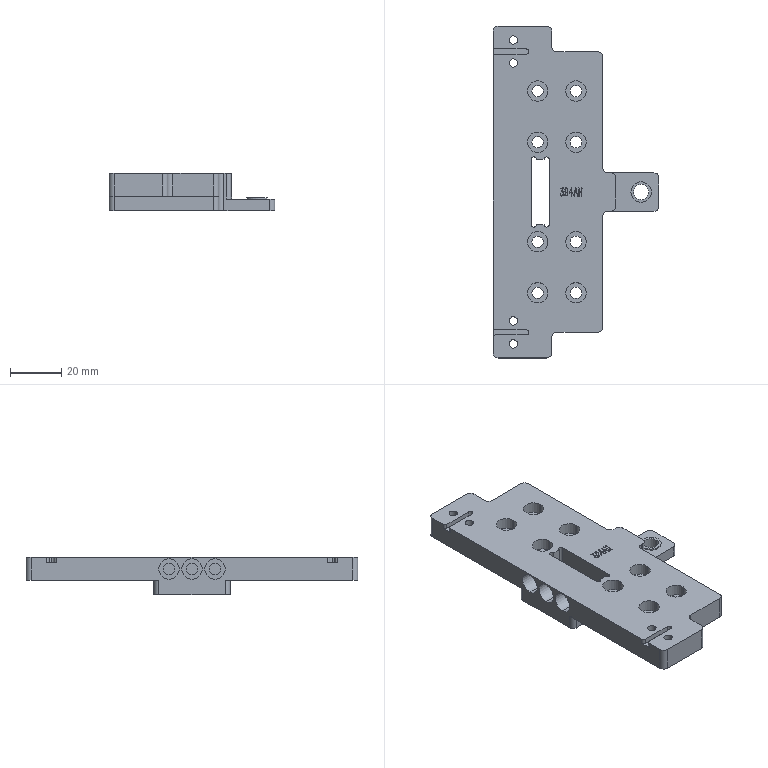NC program | NX | posted with a generic post | part box 65 x 130 x 14.5 mm
Lines 5156 to 6113 of 11541:
(PLANAR_MILL_COPY , TOOL : D2)
N10268 T20 M6
N10270 G54
N10272 G17 G0 G90 X-9.768 Y16.15 B0. C0. S9500 M3
N10274 G43 Z30. H20
N10276 Z-0.1
N10278 G94 G3 X-10.568 Y16.55 R1. F1100.
N10280 G1 X-12.75
N10282 X-12.801 Y16.531
N10284 X-12.803 Y16.472
N10286 X-12.752 Y16.45
N10288 G2 X-11.8 Y15.451 R1.
N10290 G1 Y14.969
N10292 G3 X-11.4 Y14.169 R1.
N10294 G0 X-9.768 Y16.15 Z-0.2
N10296 G3 X-10.568 Y16.55 R1.
N10298 G1 X-12.75
N10300 X-12.801 Y16.531
N10302 X-12.803 Y16.472
N10304 X-12.752 Y16.45
N10306 G2 X-11.8 Y15.451 R1.
N10308 G1 Y14.969
N10310 G3 X-11.4 Y14.169 R1.
N10312 G0 X-9.768 Y16.15 Z-0.3
N10314 G3 X-10.568 Y16.55 R1.
N10316 G1 X-12.75
N10318 X-12.801 Y16.531
N10320 X-12.803 Y16.472
N10322 X-12.752 Y16.45
N10324 G2 X-11.8 Y15.451 R1.
N10326 G1 Y14.969
N10328 G3 X-11.4 Y14.169 R1.
N10330 G0 X-9.768 Y16.15 Z-0.4
N10332 G3 X-10.568 Y16.55 R1.
N10334 G1 X-12.75
N10336 X-12.801 Y16.531
N10338 X-12.803 Y16.472
N10340 X-12.752 Y16.45
N10342 G2 X-11.8 Y15.451 R1.
N10344 G1 Y14.969
N10346 G3 X-11.4 Y14.169 R1.
N10348 G0 X-9.768 Y16.15 Z-0.5
N10350 G3 X-10.568 Y16.55 R1.
N10352 G1 X-12.75
N10354 X-12.801 Y16.531
N10356 X-12.803 Y16.472
N10358 X-12.752 Y16.45
N10360 G2 X-11.8 Y15.451 R1.
N10362 G1 Y14.969
N10364 G3 X-11.4 Y14.169 R1.
N10366 G0 X-9.768 Y16.15 Z-0.6
N10368 G3 X-10.568 Y16.55 R1.
N10370 G1 X-12.75
N10372 X-12.801 Y16.531
N10374 X-12.803 Y16.472
N10376 X-12.752 Y16.45
N10378 G2 X-11.8 Y15.451 R1.
N10380 G1 Y14.969
N10382 G3 X-11.4 Y14.169 R1.
N10384 G0 X-9.768 Y16.15 Z-0.7
N10386 G3 X-10.568 Y16.55 R1.
N10388 G1 X-12.75
N10390 X-12.801 Y16.531
N10392 X-12.803 Y16.472
N10394 X-12.752 Y16.45
N10396 G2 X-11.8 Y15.451 R1.
N10398 G1 Y14.969
N10400 G3 X-11.4 Y14.169 R1.
N10402 G0 X-9.768 Y16.15 Z-0.8
N10404 G3 X-10.568 Y16.55 R1.
N10406 G1 X-12.75
N10408 X-12.801 Y16.531
N10410 X-12.803 Y16.472
N10412 X-12.752 Y16.45
N10414 G2 X-11.8 Y15.451 R1.
N10416 G1 Y14.969
N10418 G3 X-11.4 Y14.169 R1.
N10420 G0 X-9.768 Y16.15 Z-0.9
N10422 G3 X-10.568 Y16.55 R1.
N10424 G1 X-12.75
N10426 X-12.801 Y16.531
N10428 X-12.803 Y16.472
N10430 X-12.752 Y16.45
N10432 G2 X-11.8 Y15.451 R1.
N10434 G1 Y14.969
N10436 G3 X-11.4 Y14.169 R1.
N10438 G0 X-9.768 Y16.15 Z-1.
N10440 G3 X-10.568 Y16.55 R1.
N10442 G1 X-12.75
N10444 X-12.801 Y16.531
N10446 X-12.803 Y16.472
N10448 X-12.752 Y16.45
N10450 G2 X-11.8 Y15.451 R1.
N10452 G1 Y14.969
N10454 G3 X-11.4 Y14.169 R1.
N10456 G0 X-9.768 Y16.15 Z-1.1
N10458 G3 X-10.568 Y16.55 R1.
N10460 G1 X-12.75
N10462 X-12.801 Y16.531
N10464 X-12.803 Y16.472
N10466 X-12.752 Y16.45
N10468 G2 X-11.8 Y15.451 R1.
N10470 G1 Y14.969
N10472 G3 X-11.4 Y14.169 R1.
N10474 G0 X-9.768 Y16.15 Z-1.2
N10476 G3 X-10.568 Y16.55 R1.
N10478 G1 X-12.75
N10480 X-12.801 Y16.531
N10482 X-12.803 Y16.472
N10484 X-12.752 Y16.45
N10486 G2 X-11.8 Y15.451 R1.
N10488 G1 Y14.969
N10490 G3 X-11.4 Y14.169 R1.
N10492 G0 X-9.768 Y16.15 Z-1.3
N10494 G3 X-10.568 Y16.55 R1.
N10496 G1 X-12.75
N10498 X-12.801 Y16.531
N10500 X-12.803 Y16.472
N10502 X-12.752 Y16.45
N10504 G2 X-11.8 Y15.451 R1.
N10506 G1 Y14.969
N10508 G3 X-11.4 Y14.169 R1.
N10510 G0 X-9.768 Y16.15 Z-1.4
N10512 G3 X-10.568 Y16.55 R1.
N10514 G1 X-12.75
N10516 X-12.801 Y16.531
N10518 X-12.803 Y16.472
N10520 X-12.752 Y16.45
N10522 G2 X-11.8 Y15.451 R1.
N10524 G1 Y14.969
N10526 G3 X-11.4 Y14.169 R1.
N10528 G0 X-9.768 Y16.15 Z-1.5
N10530 G3 X-10.568 Y16.55 R1.
N10532 G1 X-12.75
N10534 X-12.801 Y16.531
N10536 X-12.803 Y16.472
N10538 X-12.752 Y16.45
N10540 G2 X-11.8 Y15.451 R1.
N10542 G1 Y14.969
N10544 G3 X-11.4 Y14.169 R1.
N10546 G0 X-9.768 Y16.15 Z-1.6
N10548 G3 X-10.568 Y16.55 R1.
N10550 G1 X-12.75
N10552 X-12.801 Y16.531
N10554 X-12.803 Y16.472
N10556 X-12.752 Y16.45
N10558 G2 X-11.8 Y15.451 R1.
N10560 G1 Y14.969
N10562 G3 X-11.4 Y14.169 R1.
N10564 G0 X-9.768 Y16.15 Z-1.7
N10566 G3 X-10.568 Y16.55 R1.
N10568 G1 X-12.75
N10570 X-12.801 Y16.531
N10572 X-12.803 Y16.472
N10574 X-12.752 Y16.45
N10576 G2 X-11.8 Y15.451 R1.
N10578 G1 Y14.969
N10580 G3 X-11.4 Y14.169 R1.
N10582 G0 X-9.768 Y16.15 Z-1.8
N10584 G3 X-10.568 Y16.55 R1.
N10586 G1 X-12.75
N10588 X-12.801 Y16.531
N10590 X-12.803 Y16.472
N10592 X-12.752 Y16.45
N10594 G2 X-11.8 Y15.451 R1.
N10596 G1 Y14.969
N10598 G3 X-11.4 Y14.169 R1.
N10600 G0 X-9.768 Y16.15 Z-1.9
N10602 G3 X-10.568 Y16.55 R1.
N10604 G1 X-12.75
N10606 X-12.801 Y16.531
N10608 X-12.803 Y16.472
N10610 X-12.752 Y16.45
N10612 G2 X-11.8 Y15.451 R1.
N10614 G1 Y14.969
N10616 G3 X-11.4 Y14.169 R1.
N10618 G0 X-9.768 Y16.15 Z-2.
N10620 G3 X-10.568 Y16.55 R1.
N10622 G1 X-12.75
N10624 X-12.801 Y16.531
N10626 X-12.803 Y16.472
N10628 X-12.752 Y16.45
N10630 G2 X-11.8 Y15.451 R1.
N10632 G1 Y14.969
N10634 G3 X-11.4 Y14.169 R1.
N10636 G0 X-9.768 Y16.15 Z-2.1
N10638 G3 X-10.568 Y16.55 R1.
N10640 G1 X-12.75
N10642 X-12.801 Y16.531
N10644 X-12.803 Y16.472
N10646 X-12.752 Y16.45
N10648 G2 X-11.8 Y15.451 R1.
N10650 G1 Y14.969
N10652 G3 X-11.4 Y14.169 R1.
N10654 G0 X-9.768 Y16.15 Z-2.2
N10656 G3 X-10.568 Y16.55 R1.
N10658 G1 X-12.75
N10660 X-12.801 Y16.531
N10662 X-12.803 Y16.472
N10664 X-12.752 Y16.45
N10666 G2 X-11.8 Y15.451 R1.
N10668 G1 Y14.969
N10670 G3 X-11.4 Y14.169 R1.
N10672 G0 X-9.768 Y16.15 Z-2.3
N10674 G3 X-10.568 Y16.55 R1.
N10676 G1 X-12.75
N10678 X-12.801 Y16.531
N10680 X-12.803 Y16.472
N10682 X-12.752 Y16.45
N10684 G2 X-11.8 Y15.451 R1.
N10686 G1 Y14.969
N10688 G3 X-11.4 Y14.169 R1.
N10690 G0 X-9.768 Y16.15 Z-2.4
N10692 G3 X-10.568 Y16.55 R1.
N10694 G1 X-12.75
N10696 X-12.801 Y16.531
N10698 X-12.803 Y16.472
N10700 X-12.752 Y16.45
N10702 G2 X-11.8 Y15.451 R1.
N10704 G1 Y14.969
N10706 G3 X-11.4 Y14.169 R1.
N10708 G0 X-9.768 Y16.15 Z-2.5
N10710 G3 X-10.568 Y16.55 R1.
N10712 G1 X-12.75
N10714 X-12.801 Y16.531
N10716 X-12.803 Y16.472
N10718 X-12.752 Y16.45
N10720 G2 X-11.8 Y15.451 R1.
N10722 G1 Y14.969
N10724 G3 X-11.4 Y14.169 R1.
N10726 G0 X-9.768 Y16.15 Z-2.6
N10728 G3 X-10.568 Y16.55 R1.
N10730 G1 X-12.75
N10732 X-12.801 Y16.531
N10734 X-12.803 Y16.472
N10736 X-12.752 Y16.45
N10738 G2 X-11.8 Y15.451 R1.
N10740 G1 Y14.969
N10742 G3 X-11.4 Y14.169 R1.
N10744 G0 X-9.768 Y16.15 Z-2.7
N10746 G3 X-10.568 Y16.55 R1.
N10748 G1 X-12.75
N10750 X-12.801 Y16.531
N10752 X-12.803 Y16.472
N10754 X-12.752 Y16.45
N10756 G2 X-11.8 Y15.451 R1.
N10758 G1 Y14.969
N10760 G3 X-11.4 Y14.169 R1.
N10762 G0 X-9.768 Y16.15 Z-2.8
N10764 G3 X-10.568 Y16.55 R1.
N10766 G1 X-12.75
N10768 X-12.801 Y16.531
N10770 X-12.803 Y16.472
N10772 X-12.752 Y16.45
N10774 G2 X-11.8 Y15.451 R1.
N10776 G1 Y14.969
N10778 G3 X-11.4 Y14.169 R1.
N10780 G0 X-9.768 Y16.15 Z-2.9
N10782 G3 X-10.568 Y16.55 R1.
N10784 G1 X-12.75
N10786 X-12.801 Y16.531
N10788 X-12.803 Y16.472
N10790 X-12.752 Y16.45
N10792 G2 X-11.8 Y15.451 R1.
N10794 G1 Y14.969
N10796 G3 X-11.4 Y14.169 R1.
N10798 G0 X-9.768 Y16.15 Z-3.
N10800 G3 X-10.568 Y16.55 R1.
N10802 G1 X-12.75
N10804 X-12.801 Y16.531
N10806 X-12.803 Y16.472
N10808 X-12.752 Y16.45
N10810 G2 X-11.8 Y15.451 R1.
N10812 G1 Y14.969
N10814 G3 X-11.4 Y14.169 R1.
N10816 G0 X-9.768 Y16.15 Z-3.1
N10818 G3 X-10.568 Y16.55 R1.
N10820 G1 X-12.75
N10822 X-12.801 Y16.531
N10824 X-12.803 Y16.472
N10826 X-12.752 Y16.45
N10828 G2 X-11.8 Y15.451 R1.
N10830 G1 Y14.969
N10832 G3 X-11.4 Y14.169 R1.
N10834 G0 X-9.768 Y16.15 Z-3.2
N10836 G3 X-10.568 Y16.55 R1.
N10838 G1 X-12.75
N10840 X-12.801 Y16.531
N10842 X-12.803 Y16.472
N10844 X-12.752 Y16.45
N10846 G2 X-11.8 Y15.451 R1.
N10848 G1 Y14.969
N10850 G3 X-11.4 Y14.169 R1.
N10852 G0 X-9.768 Y16.15 Z-3.3
N10854 G3 X-10.568 Y16.55 R1.
N10856 G1 X-12.75
N10858 X-12.801 Y16.531
N10860 X-12.803 Y16.472
N10862 X-12.752 Y16.45
N10864 G2 X-11.8 Y15.451 R1.
N10866 G1 Y14.969
N10868 G3 X-11.4 Y14.169 R1.
N10870 G0 X-9.768 Y16.15 Z-3.4
N10872 G3 X-10.568 Y16.55 R1.
N10874 G1 X-12.75
N10876 X-12.801 Y16.531
N10878 X-12.803 Y16.472
N10880 X-12.752 Y16.45
N10882 G2 X-11.8 Y15.451 R1.
N10884 G1 Y14.969
N10886 G3 X-11.4 Y14.169 R1.
N10888 G0 X-9.768 Y16.15 Z-3.5
N10890 G3 X-10.568 Y16.55 R1.
N10892 G1 X-12.75
N10894 X-12.801 Y16.531
N10896 X-12.803 Y16.472
N10898 X-12.752 Y16.45
N10900 G2 X-11.8 Y15.451 R1.
N10902 G1 Y14.969
N10904 G3 X-11.4 Y14.169 R1.
N10906 G0 X-9.768 Y16.15 Z-3.6
N10908 G3 X-10.568 Y16.55 R1.
N10910 G1 X-12.75
N10912 X-12.801 Y16.531
N10914 X-12.803 Y16.472
N10916 X-12.752 Y16.45
N10918 G2 X-11.8 Y15.451 R1.
N10920 G1 Y14.969
N10922 G3 X-11.4 Y14.169 R1.
N10924 G0 X-9.768 Y16.15 Z-3.7
N10926 G3 X-10.568 Y16.55 R1.
N10928 G1 X-12.75
N10930 X-12.801 Y16.531
N10932 X-12.803 Y16.472
N10934 X-12.752 Y16.45
N10936 G2 X-11.8 Y15.451 R1.
N10938 G1 Y14.969
N10940 G3 X-11.4 Y14.169 R1.
N10942 G0 X-9.768 Y16.15 Z-3.8
N10944 G3 X-10.568 Y16.55 R1.
N10946 G1 X-12.75
N10948 X-12.801 Y16.531
N10950 X-12.803 Y16.472
N10952 X-12.752 Y16.45
N10954 G2 X-11.8 Y15.451 R1.
N10956 G1 Y14.969
N10958 G3 X-11.4 Y14.169 R1.
N10960 G0 X-9.768 Y16.15 Z-3.9
N10962 G3 X-10.568 Y16.55 R1.
N10964 G1 X-12.75
N10966 X-12.801 Y16.531
N10968 X-12.803 Y16.472
N10970 X-12.752 Y16.45
N10972 G2 X-11.8 Y15.451 R1.
N10974 G1 Y14.969
N10976 G3 X-11.4 Y14.169 R1.
N10978 G0 X-9.768 Y16.15 Z-4.
N10980 G3 X-10.568 Y16.55 R1.
N10982 G1 X-12.75
N10984 X-12.801 Y16.531
N10986 X-12.803 Y16.472
N10988 X-12.752 Y16.45
N10990 G2 X-11.8 Y15.451 R1.
N10992 G1 Y14.969
N10994 G3 X-11.4 Y14.169 R1.
N10996 G0 X-9.768 Y16.15 Z-4.1
N10998 G3 X-10.568 Y16.55 R1.
N11000 G1 X-12.75
N11002 X-12.801 Y16.531
N11004 X-12.803 Y16.472
N11006 X-12.752 Y16.45
N11008 G2 X-11.8 Y15.451 R1.
N11010 G1 Y14.969
N11012 G3 X-11.4 Y14.169 R1.
N11014 G0 X-9.768 Y16.15 Z-4.2
N11016 G3 X-10.568 Y16.55 R1.
N11018 G1 X-12.75
N11020 X-12.801 Y16.531
N11022 X-12.803 Y16.472
N11024 X-12.752 Y16.45
N11026 G2 X-11.8 Y15.451 R1.
N11028 G1 Y14.969
N11030 G3 X-11.4 Y14.169 R1.
N11032 G0 X-9.768 Y16.15 Z-4.3
N11034 G3 X-10.568 Y16.55 R1.
N11036 G1 X-12.75
N11038 X-12.801 Y16.531
N11040 X-12.803 Y16.472
N11042 X-12.752 Y16.45
N11044 G2 X-11.8 Y15.451 R1.
N11046 G1 Y14.969
N11048 G3 X-11.4 Y14.169 R1.
N11050 G0 X-9.768 Y16.15 Z-4.4
N11052 G3 X-10.568 Y16.55 R1.
N11054 G1 X-12.75
N11056 X-12.801 Y16.531
N11058 X-12.803 Y16.472
N11060 X-12.752 Y16.45
N11062 G2 X-11.8 Y15.451 R1.
N11064 G1 Y14.969
N11066 G3 X-11.4 Y14.169 R1.
N11068 G0 X-9.768 Y16.15 Z-4.5
N11070 G3 X-10.568 Y16.55 R1.
N11072 G1 X-12.75
N11074 X-12.801 Y16.531
N11076 X-12.803 Y16.472
N11078 X-12.752 Y16.45
N11080 G2 X-11.8 Y15.451 R1.
N11082 G1 Y14.969
N11084 G3 X-11.4 Y14.169 R1.
N11086 G0 X-9.768 Y16.15 Z-4.6
N11088 G3 X-10.568 Y16.55 R1.
N11090 G1 X-12.75
N11092 X-12.801 Y16.531
N11094 X-12.803 Y16.472
N11096 X-12.752 Y16.45
N11098 G2 X-11.8 Y15.451 R1.
N11100 G1 Y14.969
N11102 G3 X-11.4 Y14.169 R1.
N11104 G0 X-9.768 Y16.15 Z-4.7
N11106 G3 X-10.568 Y16.55 R1.
N11108 G1 X-12.75
N11110 X-12.801 Y16.531
N11112 X-12.803 Y16.472
N11114 X-12.752 Y16.45
N11116 G2 X-11.8 Y15.451 R1.
N11118 G1 Y14.969
N11120 G3 X-11.4 Y14.169 R1.
N11122 G0 X-9.768 Y16.15 Z-4.8
N11124 G3 X-10.568 Y16.55 R1.
N11126 G1 X-12.75
N11128 X-12.801 Y16.531
N11130 X-12.803 Y16.472
N11132 X-12.752 Y16.45
N11134 G2 X-11.8 Y15.451 R1.
N11136 G1 Y14.969
N11138 G3 X-11.4 Y14.169 R1.
N11140 G0 X-9.768 Y16.15 Z-4.9
N11142 G3 X-10.568 Y16.55 R1.
N11144 G1 X-12.75
N11146 X-12.801 Y16.531
N11148 X-12.803 Y16.472
N11150 X-12.752 Y16.45
N11152 G2 X-11.8 Y15.451 R1.
N11154 G1 Y14.969
N11156 G3 X-11.4 Y14.169 R1.
N11158 G0 X-9.768 Y16.15 Z-5.
N11160 G3 X-10.568 Y16.55 R1.
N11162 G1 X-12.75
N11164 X-12.801 Y16.531
N11166 X-12.803 Y16.472
N11168 X-12.752 Y16.45
N11170 G2 X-11.8 Y15.451 R1.
N11172 G1 Y14.969
N11174 G3 X-11.4 Y14.169 R1.
N11176 G0 X-9.768 Y16.15 Z-5.1
N11178 G3 X-10.568 Y16.55 R1.
N11180 G1 X-12.75
N11182 X-12.801 Y16.531
N11184 X-12.803 Y16.472
N11186 X-12.752 Y16.45
N11188 G2 X-11.8 Y15.451 R1.
N11190 G1 Y14.969
N11192 G3 X-11.4 Y14.169 R1.
N11194 G0 X-9.768 Y16.15 Z-5.2
N11196 G3 X-10.568 Y16.55 R1.
N11198 G1 X-12.75
N11200 X-12.801 Y16.531
N11202 X-12.803 Y16.472
N11204 X-12.752 Y16.45
N11206 G2 X-11.8 Y15.451 R1.
N11208 G1 Y14.969
N11210 G3 X-11.4 Y14.169 R1.
N11212 G0 X-9.768 Y16.15 Z-5.3
N11214 G3 X-10.568 Y16.55 R1.
N11216 G1 X-12.75
N11218 X-12.801 Y16.531
N11220 X-12.803 Y16.472
N11222 X-12.752 Y16.45
N11224 G2 X-11.8 Y15.451 R1.
N11226 G1 Y14.969
N11228 G3 X-11.4 Y14.169 R1.
N11230 G0 X-9.768 Y16.15 Z-5.4
N11232 G3 X-10.568 Y16.55 R1.
N11234 G1 X-12.75
N11236 X-12.801 Y16.531
N11238 X-12.803 Y16.472
N11240 X-12.752 Y16.45
N11242 G2 X-11.8 Y15.451 R1.
N11244 G1 Y14.969
N11246 G3 X-11.4 Y14.169 R1.
N11248 G0 X-9.768 Y16.15 Z-5.5
N11250 G3 X-10.568 Y16.55 R1.
N11252 G1 X-12.75
N11254 X-12.801 Y16.531
N11256 X-12.803 Y16.472
N11258 X-12.752 Y16.45
N11260 G2 X-11.8 Y15.451 R1.
N11262 G1 Y14.969
N11264 G3 X-11.4 Y14.169 R1.
N11266 G0 X-9.768 Y16.15 Z-5.6
N11268 G3 X-10.568 Y16.55 R1.
N11270 G1 X-12.75
N11272 X-12.801 Y16.531
N11274 X-12.803 Y16.472
N11276 X-12.752 Y16.45
N11278 G2 X-11.8 Y15.451 R1.
N11280 G1 Y14.969
N11282 G3 X-11.4 Y14.169 R1.
N11284 G0 X-9.768 Y16.15 Z-5.7
N11286 G3 X-10.568 Y16.55 R1.
N11288 G1 X-12.75
N11290 X-12.801 Y16.531
N11292 X-12.803 Y16.472
N11294 X-12.752 Y16.45
N11296 G2 X-11.8 Y15.451 R1.
N11298 G1 Y14.969
N11300 G3 X-11.4 Y14.169 R1.
N11302 G0 X-9.768 Y16.15 Z-5.8
N11304 G3 X-10.568 Y16.55 R1.
N11306 G1 X-12.75
N11308 X-12.801 Y16.531
N11310 X-12.803 Y16.472
N11312 X-12.752 Y16.45
N11314 G2 X-11.8 Y15.451 R1.
N11316 G1 Y14.969
N11318 G3 X-11.4 Y14.169 R1.
N11320 G0 X-9.768 Y16.15 Z-5.9
N11322 G3 X-10.568 Y16.55 R1.
N11324 G1 X-12.75
N11326 X-12.801 Y16.531
N11328 X-12.803 Y16.472
N11330 X-12.752 Y16.45
N11332 G2 X-11.8 Y15.451 R1.
N11334 G1 Y14.969
N11336 G3 X-11.4 Y14.169 R1.
N11338 G0 X-9.768 Y16.15 Z-6.
N11340 G3 X-10.568 Y16.55 R1.
N11342 G1 X-12.75
N11344 X-12.801 Y16.531
N11346 X-12.803 Y16.472
N11348 X-12.752 Y16.45
N11350 G2 X-11.8 Y15.451 R1.
N11352 G1 Y14.969
N11354 G3 X-11.4 Y14.169 R1.
N11356 G0 X-9.768 Y16.15 Z-6.1
N11358 G3 X-10.568 Y16.55 R1.
N11360 G1 X-12.75
N11362 X-12.801 Y16.531
N11364 X-12.803 Y16.472
N11366 X-12.752 Y16.45
N11368 G2 X-11.8 Y15.451 R1.
N11370 G1 Y14.969
N11372 G3 X-11.4 Y14.169 R1.
N11374 G0 X-9.768 Y16.15 Z-6.2
N11376 G3 X-10.568 Y16.55 R1.
N11378 G1 X-12.75
N11380 X-12.801 Y16.531
N11382 X-12.803 Y16.472
N11384 X-12.752 Y16.45
N11386 G2 X-11.8 Y15.451 R1.
N11388 G1 Y14.969
N11390 G3 X-11.4 Y14.169 R1.
N11392 G0 X-9.768 Y16.15 Z-6.3
N11394 G3 X-10.568 Y16.55 R1.
N11396 G1 X-12.75
N11398 X-12.801 Y16.531
N11400 X-12.803 Y16.472
N11402 X-12.752 Y16.45
N11404 G2 X-11.8 Y15.451 R1.
N11406 G1 Y14.969
N11408 G3 X-11.4 Y14.169 R1.
N11410 G0 X-9.768 Y16.15 Z-6.4
N11412 G3 X-10.568 Y16.55 R1.
N11414 G1 X-12.75
N11416 X-12.801 Y16.531
N11418 X-12.803 Y16.472
N11420 X-12.752 Y16.45
N11422 G2 X-11.8 Y15.451 R1.
N11424 G1 Y14.969
N11426 G3 X-11.4 Y14.169 R1.
N11428 G0 X-9.768 Y16.15 Z-6.5
N11430 G3 X-10.568 Y16.55 R1.
N11432 G1 X-12.75
N11434 X-12.801 Y16.531
N11436 X-12.803 Y16.472
N11438 X-12.752 Y16.45
N11440 G2 X-11.8 Y15.451 R1.
N11442 G1 Y14.969
N11444 G3 X-11.4 Y14.169 R1.
N11446 G0 X-9.768 Y16.15 Z-6.6
N11448 G3 X-10.568 Y16.55 R1.
N11450 G1 X-12.75
N11452 X-12.801 Y16.531
N11454 X-12.803 Y16.472
N11456 X-12.752 Y16.45
N11458 G2 X-11.8 Y15.451 R1.
N11460 G1 Y14.969
N11462 G3 X-11.4 Y14.169 R1.
N11464 G0 X-9.768 Y16.15 Z-6.7
N11466 G3 X-10.568 Y16.55 R1.
N11468 G1 X-12.75
N11470 X-12.801 Y16.531
N11472 X-12.803 Y16.472
N11474 X-12.752 Y16.45
N11476 G2 X-11.8 Y15.451 R1.
N11478 G1 Y14.969
N11480 G3 X-11.4 Y14.169 R1.
N11482 G0 X-9.768 Y16.15 Z-6.8
N11484 G3 X-10.568 Y16.55 R1.
N11486 G1 X-12.75
N11488 X-12.801 Y16.531
N11490 X-12.803 Y16.472
N11492 X-12.752 Y16.45
N11494 G2 X-11.8 Y15.451 R1.
N11496 G1 Y14.969
N11498 G3 X-11.4 Y14.169 R1.
N11500 G0 X-9.768 Y16.15 Z-6.9
N11502 G3 X-10.568 Y16.55 R1.
N11504 G1 X-12.75
N11506 X-12.801 Y16.531
N11508 X-12.803 Y16.472
N11510 X-12.752 Y16.45
N11512 G2 X-11.8 Y15.451 R1.
N11514 G1 Y14.969
N11516 G3 X-11.4 Y14.169 R1.
N11518 G0 X-9.768 Y16.15 Z-7.
N11520 G3 X-10.568 Y16.55 R1.
N11522 G1 X-12.75
N11524 X-12.801 Y16.531
N11526 X-12.803 Y16.472
N11528 X-12.752 Y16.45
N11530 G2 X-11.8 Y15.451 R1.
N11532 G1 Y14.969
N11534 G3 X-11.4 Y14.169 R1.
N11536 G0 X-9.768 Y16.15 Z-7.1
N11538 G3 X-10.568 Y16.55 R1.
N11540 G1 X-12.75
N11542 X-12.801 Y16.531
N11544 X-12.803 Y16.472
N11546 X-12.752 Y16.45
N11548 G2 X-11.8 Y15.451 R1.
N11550 G1 Y14.969
N11552 G3 X-11.4 Y14.169 R1.
N11554 G0 X-9.768 Y16.15 Z-7.2
N11556 G3 X-10.568 Y16.55 R1.
N11558 G1 X-12.75
N11560 X-12.801 Y16.531
N11562 X-12.803 Y16.472
N11564 X-12.752 Y16.45
N11566 G2 X-11.8 Y15.451 R1.
N11568 G1 Y14.969
N11570 G3 X-11.4 Y14.169 R1.
N11572 G0 X-9.768 Y16.15 Z-7.3
N11574 G3 X-10.568 Y16.55 R1.
N11576 G1 X-12.75
N11578 X-12.801 Y16.531
N11580 X-12.803 Y16.472
N11582 X-12.752 Y16.45
N11584 G2 X-11.8 Y15.451 R1.
N11586 G1 Y14.969
N11588 G3 X-11.4 Y14.169 R1.
N11590 G0 X-9.768 Y16.15 Z-7.4
N11592 G3 X-10.568 Y16.55 R1.
N11594 G1 X-12.75
N11596 X-12.801 Y16.531
N11598 X-12.803 Y16.472
N11600 X-12.752 Y16.45
N11602 G2 X-11.8 Y15.451 R1.
N11604 G1 Y14.969
N11606 G3 X-11.4 Y14.169 R1.
N11608 G0 X-9.768 Y16.15 Z-7.5
N11610 G3 X-10.568 Y16.55 R1.
N11612 G1 X-12.75
N11614 X-12.801 Y16.531
N11616 X-12.803 Y16.472
N11618 X-12.752 Y16.45
N11620 G2 X-11.8 Y15.451 R1.
N11622 G1 Y14.969
N11624 G3 X-11.4 Y14.169 R1.
N11626 G0 X-9.768 Y16.15 Z-7.6
N11628 G3 X-10.568 Y16.55 R1.
N11630 G1 X-12.75
N11632 X-12.801 Y16.531
N11634 X-12.803 Y16.472
N11636 X-12.752 Y16.45
N11638 G2 X-11.8 Y15.451 R1.
N11640 G1 Y14.969
N11642 G3 X-11.4 Y14.169 R1.
N11644 G0 X-9.768 Y16.15 Z-7.7
N11646 G3 X-10.568 Y16.55 R1.
N11648 G1 X-12.75
N11650 X-12.801 Y16.531
N11652 X-12.803 Y16.472
N11654 X-12.752 Y16.45
N11656 G2 X-11.8 Y15.451 R1.
N11658 G1 Y14.969
N11660 G3 X-11.4 Y14.169 R1.
N11662 G0 X-9.768 Y16.15 Z-7.8
N11664 G3 X-10.568 Y16.55 R1.
N11666 G1 X-12.75
N11668 X-12.801 Y16.531
N11670 X-12.803 Y16.472
N11672 X-12.752 Y16.45
N11674 G2 X-11.8 Y15.451 R1.
N11676 G1 Y14.969
N11678 G3 X-11.4 Y14.169 R1.
N11680 G0 X-9.768 Y16.15 Z-7.9
N11682 G3 X-10.568 Y16.55 R1.
N11684 G1 X-12.75
N11686 X-12.801 Y16.531
N11688 X-12.803 Y16.472
N11690 X-12.752 Y16.45
N11692 G2 X-11.8 Y15.451 R1.
N11694 G1 Y14.969
N11696 G3 X-11.4 Y14.169 R1.
N11698 G0 X-9.768 Y16.15 Z-8.
N11700 G3 X-10.568 Y16.55 R1.
N11702 G1 X-12.75
N11704 X-12.801 Y16.531
N11706 X-12.803 Y16.472
N11708 X-12.752 Y16.45
N11710 G2 X-11.8 Y15.451 R1.
N11712 G1 Y14.969
N11714 G3 X-11.4 Y14.169 R1.
N11716 G0 X-9.768 Y16.15 Z-8.1
N11718 G3 X-10.568 Y16.55 R1.
N11720 G1 X-12.75
N11722 X-12.801 Y16.531
N11724 X-12.803 Y16.472
N11726 X-12.752 Y16.45
N11728 G2 X-11.8 Y15.451 R1.
N11730 G1 Y14.969
N11732 G3 X-11.4 Y14.169 R1.
N11734 G0 X-9.768 Y16.15 Z-8.2
N11736 G3 X-10.568 Y16.55 R1.
N11738 G1 X-12.75
N11740 X-12.801 Y16.531
N11742 X-12.803 Y16.472
N11744 X-12.752 Y16.45
N11746 G2 X-11.8 Y15.451 R1.
N11748 G1 Y14.969
N11750 G3 X-11.4 Y14.169 R1.
N11752 G0 X-9.768 Y16.15 Z-8.3
N11754 G3 X-10.568 Y16.55 R1.
N11756 G1 X-12.75
N11758 X-12.801 Y16.531
N11760 X-12.803 Y16.472
N11762 X-12.752 Y16.45
N11764 G2 X-11.8 Y15.451 R1.
N11766 G1 Y14.969
N11768 G3 X-11.4 Y14.169 R1.
N11770 G0 X-9.768 Y16.15 Z-8.4
N11772 G3 X-10.568 Y16.55 R1.
N11774 G1 X-12.75
N11776 X-12.801 Y16.531
N11778 X-12.803 Y16.472
N11780 X-12.752 Y16.45
N11782 G2 X-11.8 Y15.451 R1.
N11784 G1 Y14.969
N11786 G3 X-11.4 Y14.169 R1.
N11788 G0 X-9.768 Y16.15 Z-8.5
N11790 G3 X-10.568 Y16.55 R1.
N11792 G1 X-12.75
N11794 X-12.801 Y16.531
N11796 X-12.803 Y16.472
N11798 X-12.752 Y16.45
N11800 G2 X-11.8 Y15.451 R1.
N11802 G1 Y14.969
N11804 G3 X-11.4 Y14.169 R1.
N11806 G0 X-9.768 Y16.15 Z-8.6
N11808 G3 X-10.568 Y16.55 R1.
N11810 G1 X-12.75
N11812 X-12.801 Y16.531
N11814 X-12.803 Y16.472
N11816 X-12.752 Y16.45
N11818 G2 X-11.8 Y15.451 R1.
N11820 G1 Y14.969
N11822 G3 X-11.4 Y14.169 R1.
N11824 G0 X-9.768 Y16.15 Z-8.7
N11826 G3 X-10.568 Y16.55 R1.
N11828 G1 X-12.75
N11830 X-12.801 Y16.531
N11832 X-12.803 Y16.472
N11834 X-12.752 Y16.45
N11836 G2 X-11.8 Y15.451 R1.
N11838 G1 Y14.969
N11840 G3 X-11.4 Y14.169 R1.
N11842 G0 X-9.768 Y16.15 Z-8.8
N11844 G3 X-10.568 Y16.55 R1.
N11846 G1 X-12.75
N11848 X-12.801 Y16.531
N11850 X-12.803 Y16.472
N11852 X-12.752 Y16.45
N11854 G2 X-11.8 Y15.451 R1.
N11856 G1 Y14.969
N11858 G3 X-11.4 Y14.169 R1.
N11860 G0 X-9.768 Y16.15 Z-8.9
N11862 G3 X-10.568 Y16.55 R1.
N11864 G1 X-12.75
N11866 X-12.801 Y16.531
N11868 X-12.803 Y16.472
N11870 X-12.752 Y16.45
N11872 G2 X-11.8 Y15.451 R1.
N11874 G1 Y14.969
N11876 G3 X-11.4 Y14.169 R1.
N11878 G0 X-9.768 Y16.15 Z-9.
N11880 G3 X-10.568 Y16.55 R1.
N11882 G1 X-12.75
N11884 X-12.801 Y16.531
N11886 X-12.803 Y16.472
N11888 X-12.752 Y16.45
N11890 G2 X-11.8 Y15.451 R1.
N11892 G1 Y14.969
N11894 G3 X-11.4 Y14.169 R1.
N11896 G0 X-9.768 Y16.15 Z-9.1
N11898 G3 X-10.568 Y16.55 R1.
N11900 G1 X-12.75
N11902 X-12.801 Y16.531
N11904 X-12.803 Y16.472
N11906 X-12.752 Y16.45
N11908 G2 X-11.8 Y15.451 R1.
N11910 G1 Y14.969
N11912 G3 X-11.4 Y14.169 R1.
N11914 G0 X-9.768 Y16.15 Z-9.2
N11916 G3 X-10.568 Y16.55 R1.
N11918 G1 X-12.75
N11920 X-12.801 Y16.531
N11922 X-12.803 Y16.472
N11924 X-12.752 Y16.45
N11926 G2 X-11.8 Y15.451 R1.
N11928 G1 Y14.969
N11930 G3 X-11.4 Y14.169 R1.
N11932 G0 X-9.768 Y16.15 Z-9.3
N11934 G3 X-10.568 Y16.55 R1.
N11936 G1 X-12.75
N11938 X-12.801 Y16.531
N11940 X-12.803 Y16.472
N11942 X-12.752 Y16.45
N11944 G2 X-11.8 Y15.451 R1.
N11946 G1 Y14.969
N11948 G3 X-11.4 Y14.169 R1.
N11950 G0 X-9.768 Y16.15 Z-9.4
N11952 G3 X-10.568 Y16.55 R1.
N11954 G1 X-12.75
N11956 X-12.801 Y16.531
N11958 X-12.803 Y16.472
N11960 X-12.752 Y16.45
N11962 G2 X-11.8 Y15.451 R1.
N11964 G1 Y14.969
N11966 G3 X-11.4 Y14.169 R1.
N11968 G0 X-9.768 Y16.15 Z-9.5
N11970 G3 X-10.568 Y16.55 R1.
N11972 G1 X-12.75
N11974 X-12.801 Y16.531
N11976 X-12.803 Y16.472
N11978 X-12.752 Y16.45
N11980 G2 X-11.8 Y15.451 R1.
N11982 G1 Y14.969
N11984 G3 X-11.4 Y14.169 R1.
N11986 G0 X-9.768 Y16.15 Z-9.6
N11988 G3 X-10.568 Y16.55 R1.
N11990 G1 X-12.75
N11992 X-12.801 Y16.531
N11994 X-12.803 Y16.472
N11996 X-12.752 Y16.45
N11998 G2 X-11.8 Y15.451 R1.
N12000 G1 Y14.969
N12002 G3 X-11.4 Y14.169 R1.
N12004 G0 X-9.768 Y16.15 Z-9.7
N12006 G3 X-10.568 Y16.55 R1.
N12008 G1 X-12.75
N12010 X-12.801 Y16.531
N12012 X-12.803 Y16.472
N12014 X-12.752 Y16.45
N12016 G2 X-11.8 Y15.451 R1.
N12018 G1 Y14.969
N12020 G3 X-11.4 Y14.169 R1.
N12022 G0 X-9.768 Y16.15 Z-9.8
N12024 G3 X-10.568 Y16.55 R1.
N12026 G1 X-12.75
N12028 X-12.801 Y16.531
N12030 X-12.803 Y16.472
N12032 X-12.752 Y16.45
N12034 G2 X-11.8 Y15.451 R1.
N12036 G1 Y14.969
N12038 G3 X-11.4 Y14.169 R1.
N12040 G0 X-9.768 Y16.15 Z-9.9
N12042 G3 X-10.568 Y16.55 R1.
N12044 G1 X-12.75
N12046 X-12.801 Y16.531
N12048 X-12.803 Y16.472
N12050 X-12.752 Y16.45
N12052 G2 X-11.8 Y15.451 R1.
N12054 G1 Y14.969
N12056 G3 X-11.4 Y14.169 R1.
N12058 G0 X-9.768 Y16.15 Z-10.
N12060 G3 X-10.568 Y16.55 R1.
N12062 G1 X-12.75
N12064 X-12.801 Y16.531
N12066 X-12.803 Y16.472
N12068 X-12.752 Y16.45
N12070 G2 X-11.8 Y15.451 R1.
N12072 G1 Y14.969
N12074 G3 X-11.4 Y14.169 R1.
N12076 G0 X-9.768 Y16.15 Z-10.1
N12078 G3 X-10.568 Y16.55 R1.
N12080 G1 X-12.75
N12082 X-12.801 Y16.531
N12084 X-12.803 Y16.472
N12086 X-12.752 Y16.45
N12088 G2 X-11.8 Y15.451 R1.
N12090 G1 Y14.969
N12092 G3 X-11.4 Y14.169 R1.
N12094 G0 X-9.768 Y16.15 Z-10.2
N12096 G3 X-10.568 Y16.55 R1.
N12098 G1 X-12.75
N12100 X-12.801 Y16.531
N12102 X-12.803 Y16.472
N12104 X-12.752 Y16.45
N12106 G2 X-11.8 Y15.451 R1.
N12108 G1 Y14.969
N12110 G3 X-11.4 Y14.169 R1.
N12112 G0 X-9.768 Y16.15 Z-10.3
N12114 G3 X-10.568 Y16.55 R1.
N12116 G1 X-12.75
N12118 X-12.801 Y16.531
N12120 X-12.803 Y16.472
N12122 X-12.752 Y16.45
N12124 G2 X-11.8 Y15.451 R1.
N12126 G1 Y14.969
N12128 G3 X-11.4 Y14.169 R1.
N12130 G0 X-9.768 Y16.15 Z-10.4
N12132 G3 X-10.568 Y16.55 R1.
N12134 G1 X-12.75
N12136 X-12.801 Y16.531
N12138 X-12.803 Y16.472
N12140 X-12.752 Y16.45
N12142 G2 X-11.8 Y15.451 R1.
N12144 G1 Y14.969
N12146 G3 X-11.4 Y14.169 R1.
N12148 G0 X-9.768 Y16.15 Z-10.5
N12150 G3 X-10.568 Y16.55 R1.
N12152 G1 X-12.75
N12154 X-12.801 Y16.531
N12156 X-12.803 Y16.472
N12158 X-12.752 Y16.45
N12160 G2 X-11.8 Y15.451 R1.
N12162 G1 Y14.969
N12164 G3 X-11.4 Y14.169 R1.
N12166 G0 X-9.768 Y16.15 Z-10.6
N12168 G3 X-10.568 Y16.55 R1.
N12170 G1 X-12.75
N12172 X-12.801 Y16.531
N12174 X-12.803 Y16.472
N12176 X-12.752 Y16.45